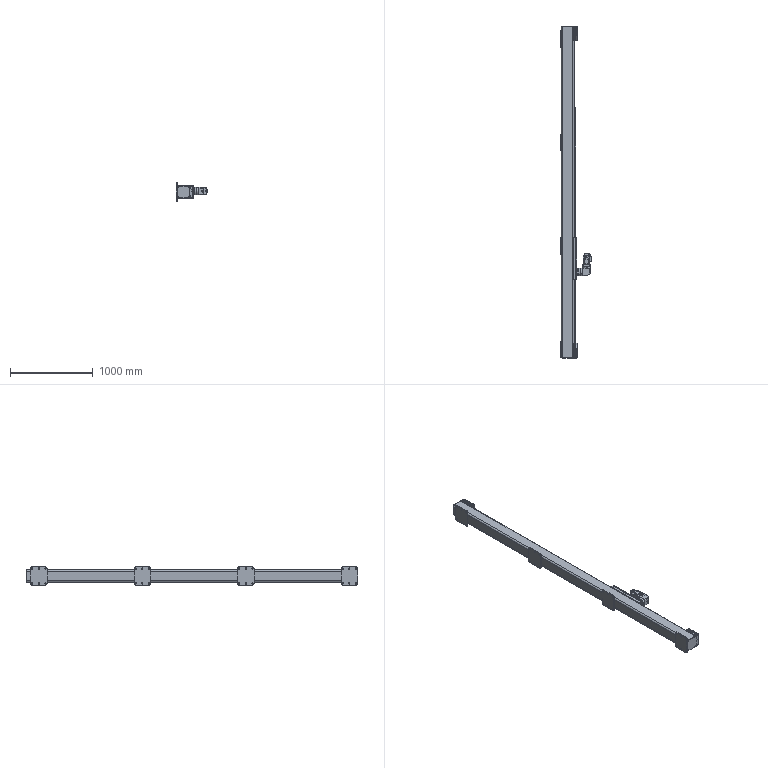Part | SolidWorks | features ReferencePattern 8, LocalLPattern 2, MirrorCompFeat 2 | 41 solids | 12170 faces | volume 25579409 mm3 | plane 7998 | cylinder 2114 | spline 1716 | torus 142 | sphere 118 | cone 82 | commonest cylinder face diameters 4.5 x328 5.2 x268 7.5 x268 1 x116 4 x78 3.3 x76